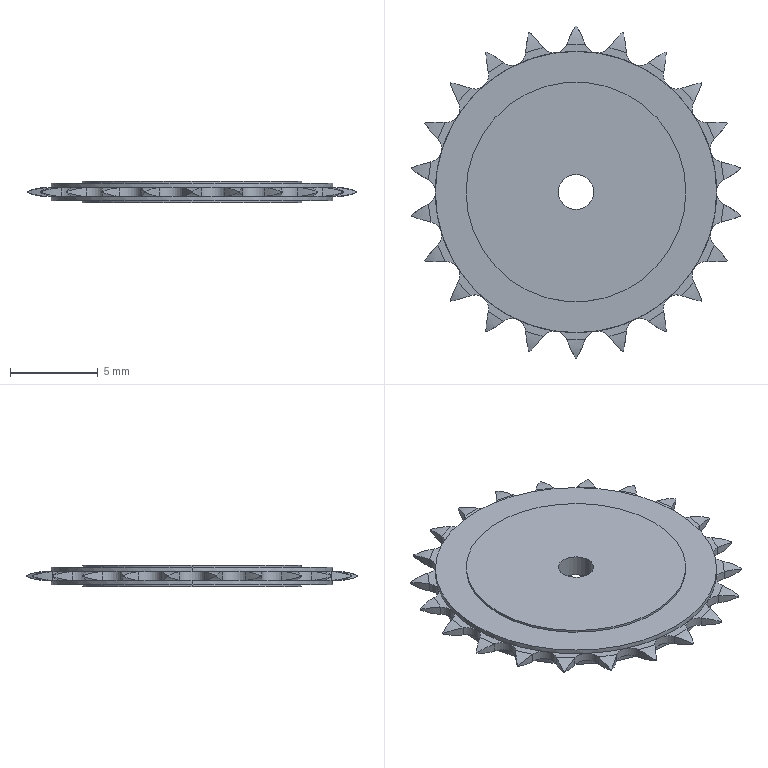Part | SolidWorks | features ICE 4, Scale 3, CirPattern 1, Extrusion 1 | 1 solid | 190 faces | box 18.705 x 18.888 x 1.25 mm | volume 239.549 mm3 | cylinder 120 | plane 70 | commonest cylinder face diameters 6.25 x44 15.224 x44 1.567 x22 12.5 x4 16 x4 2 x2